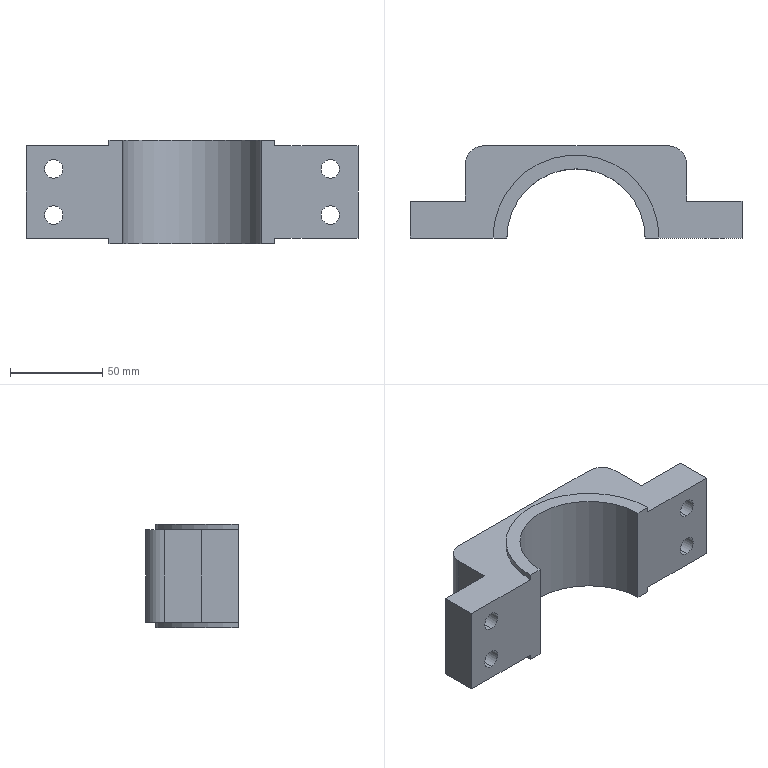Part | SolidWorks | features ICE 4, Extrusion 1, Fillet 1, MirrorPattern 1 | 1 solid | 26 faces | box 180 x 50 x 56 mm | volume 246956 mm3 | cylinder 13 | plane 13 | commonest cylinder face diameters 10 x8 20 x2 90 x2 75 x1
STEP:
#1=CARTESIAN_POINT('',(-75.,0.,17.5));
#2=VERTEX_POINT('',#1);
#3=CARTESIAN_POINT('',(-75.,0.,7.5));
#4=VERTEX_POINT('',#3);
#5=CARTESIAN_POINT('',(-75.,0.,12.5));
#6=DIRECTION('',(0.,-1.,0.));
#7=DIRECTION('',(0.,0.,-1.));
#8=AXIS2_PLACEMENT_3D('',#5,#6,#7);
#9=CIRCLE('',#8,5.);
#10=EDGE_CURVE('',#2,#4,#9,.T.);
#11=ORIENTED_EDGE('',*,*,#10,.T.);
#12=CARTESIAN_POINT('',(-75.,20.,7.5));
#13=VERTEX_POINT('',#12);
#14=CARTESIAN_POINT('',(-75.,-18.,7.5));
#15=DIRECTION('',(0.,1.,0.));
#16=VECTOR('',#15,1000.);
#17=LINE('',#14,#16);
#18=EDGE_CURVE('',#4,#13,#17,.T.);
#19=ORIENTED_EDGE('',*,*,#18,.T.);
#20=CARTESIAN_POINT('',(-75.,20.,17.5));
#21=VERTEX_POINT('',#20);
#22=CARTESIAN_POINT('',(-75.,20.,12.5));
#23=DIRECTION('',(0.,1.,0.));
#24=DIRECTION('',(0.,0.,1.));
#25=AXIS2_PLACEMENT_3D('',#22,#23,#24);
#26=CIRCLE('',#25,5.);
#27=EDGE_CURVE('',#13,#21,#26,.T.);
#28=ORIENTED_EDGE('',*,*,#27,.T.);
#29=CARTESIAN_POINT('',(-75.,-18.,17.5));
#30=DIRECTION('',(0.,1.,0.));
#31=VECTOR('',#30,1000.);
#32=LINE('',#29,#31);
#33=EDGE_CURVE('',#2,#21,#32,.T.);
#34=ORIENTED_EDGE('',*,*,#33,.F.);
#35=EDGE_LOOP('',(#11,#19,#28,#34));
#36=FACE_OUTER_BOUND('',#35,.T.);
#37=CARTESIAN_POINT('',(-75.,-18.,12.5));
#38=DIRECTION('',(0.,1.,0.));
#39=DIRECTION('',(0.,0.,1.));
#40=AXIS2_PLACEMENT_3D('',#37,#38,#39);
#41=CYLINDRICAL_SURFACE('',#40,5.);
#42=ADVANCED_FACE('',(#36),#41,.F.);
#43=CARTESIAN_POINT('',(-75.,0.,-7.5));
#44=VERTEX_POINT('',#43);
#45=CARTESIAN_POINT('',(-75.,0.,-17.5));
#46=VERTEX_POINT('',#45);
#47=CARTESIAN_POINT('',(-75.,0.,-12.5));
#48=DIRECTION('',(0.,-1.,0.));
#49=DIRECTION('',(0.,0.,-1.));
#50=AXIS2_PLACEMENT_3D('',#47,#48,#49);
#51=CIRCLE('',#50,5.);
#52=EDGE_CURVE('',#44,#46,#51,.T.);
#53=ORIENTED_EDGE('',*,*,#52,.T.);
#54=CARTESIAN_POINT('',(-75.,20.,-17.5));
#55=VERTEX_POINT('',#54);
#56=CARTESIAN_POINT('',(-75.,-18.,-17.5));
#57=DIRECTION('',(0.,1.,0.));
#58=VECTOR('',#57,1000.);
#59=LINE('',#56,#58);
#60=EDGE_CURVE('',#46,#55,#59,.T.);
#61=ORIENTED_EDGE('',*,*,#60,.T.);
#62=CARTESIAN_POINT('',(-75.,20.,-7.5));
#63=VERTEX_POINT('',#62);
#64=CARTESIAN_POINT('',(-75.,20.,-12.5));
#65=DIRECTION('',(0.,1.,0.));
#66=DIRECTION('',(0.,0.,1.));
#67=AXIS2_PLACEMENT_3D('',#64,#65,#66);
#68=CIRCLE('',#67,5.);
#69=EDGE_CURVE('',#55,#63,#68,.T.);
#70=ORIENTED_EDGE('',*,*,#69,.T.);
#71=CARTESIAN_POINT('',(-75.,-18.,-7.5));
#72=DIRECTION('',(0.,1.,0.));
#73=VECTOR('',#72,1000.);
#74=LINE('',#71,#73);
#75=EDGE_CURVE('',#44,#63,#74,.T.);
#76=ORIENTED_EDGE('',*,*,#75,.F.);
#77=EDGE_LOOP('',(#53,#61,#70,#76));
#78=FACE_OUTER_BOUND('',#77,.T.);
#79=CARTESIAN_POINT('',(-75.,-18.,-12.5));
#80=DIRECTION('',(0.,1.,0.));
#81=DIRECTION('',(0.,0.,1.));
#82=AXIS2_PLACEMENT_3D('',#79,#80,#81);
#83=CYLINDRICAL_SURFACE('',#82,5.);
#84=ADVANCED_FACE('',(#78),#83,.F.);
#85=CARTESIAN_POINT('',(75.,0.,-7.5));
#86=VERTEX_POINT('',#85);
#87=CARTESIAN_POINT('',(75.,0.,-17.5));
#88=VERTEX_POINT('',#87);
#89=CARTESIAN_POINT('',(75.,0.,-12.5));
#90=DIRECTION('',(0.,-1.,0.));
#91=DIRECTION('',(0.,0.,-1.));
#92=AXIS2_PLACEMENT_3D('',#89,#90,#91);
#93=CIRCLE('',#92,5.);
#94=EDGE_CURVE('',#86,#88,#93,.T.);
#95=ORIENTED_EDGE('',*,*,#94,.T.);
#96=CARTESIAN_POINT('',(75.,20.,-17.5));
#97=VERTEX_POINT('',#96);
#98=CARTESIAN_POINT('',(75.,-18.,-17.5));
#99=DIRECTION('',(0.,1.,0.));
#100=VECTOR('',#99,1000.);
#101=LINE('',#98,#100);
#102=EDGE_CURVE('',#88,#97,#101,.T.);
#103=ORIENTED_EDGE('',*,*,#102,.T.);
#104=CARTESIAN_POINT('',(75.,20.,-7.5));
#105=VERTEX_POINT('',#104);
#106=CARTESIAN_POINT('',(75.,20.,-12.5));
#107=DIRECTION('',(0.,1.,0.));
#108=DIRECTION('',(0.,0.,-1.));
#109=AXIS2_PLACEMENT_3D('',#106,#107,#108);
#110=CIRCLE('',#109,5.);
#111=EDGE_CURVE('',#97,#105,#110,.T.);
#112=ORIENTED_EDGE('',*,*,#111,.T.);
#113=CARTESIAN_POINT('',(75.,-18.,-7.5));
#114=DIRECTION('',(0.,1.,0.));
#115=VECTOR('',#114,1000.);
#116=LINE('',#113,#115);
#117=EDGE_CURVE('',#86,#105,#116,.T.);
#118=ORIENTED_EDGE('',*,*,#117,.F.);
#119=EDGE_LOOP('',(#95,#103,#112,#118));
#120=FACE_OUTER_BOUND('',#119,.T.);
#121=CARTESIAN_POINT('',(75.,-18.,-12.5));
#122=DIRECTION('',(0.,1.,0.));
#123=DIRECTION('',(0.,0.,1.));
#124=AXIS2_PLACEMENT_3D('',#121,#122,#123);
#125=CYLINDRICAL_SURFACE('',#124,5.);
#126=ADVANCED_FACE('',(#120),#125,.F.);
#127=CARTESIAN_POINT('',(75.,0.,17.5));
#128=VERTEX_POINT('',#127);
#129=CARTESIAN_POINT('',(75.,0.,7.5));
#130=VERTEX_POINT('',#129);
#131=CARTESIAN_POINT('',(75.,0.,12.5));
#132=DIRECTION('',(0.,-1.,0.));
#133=DIRECTION('',(0.,0.,-1.));
#134=AXIS2_PLACEMENT_3D('',#131,#132,#133);
#135=CIRCLE('',#134,5.);
#136=EDGE_CURVE('',#128,#130,#135,.T.);
#137=ORIENTED_EDGE('',*,*,#136,.T.);
#138=CARTESIAN_POINT('',(75.,20.,7.5));
#139=VERTEX_POINT('',#138);
#140=CARTESIAN_POINT('',(75.,-18.,7.5));
#141=DIRECTION('',(0.,1.,0.));
#142=VECTOR('',#141,1000.);
#143=LINE('',#140,#142);
#144=EDGE_CURVE('',#130,#139,#143,.T.);
#145=ORIENTED_EDGE('',*,*,#144,.T.);
#146=CARTESIAN_POINT('',(75.,20.,17.5));
#147=VERTEX_POINT('',#146);
#148=CARTESIAN_POINT('',(75.,20.,12.5));
#149=DIRECTION('',(0.,1.,0.));
#150=DIRECTION('',(0.,0.,-1.));
#151=AXIS2_PLACEMENT_3D('',#148,#149,#150);
#152=CIRCLE('',#151,5.);
#153=EDGE_CURVE('',#139,#147,#152,.T.);
#154=ORIENTED_EDGE('',*,*,#153,.T.);
#155=CARTESIAN_POINT('',(75.,-18.,17.5));
#156=DIRECTION('',(0.,1.,0.));
#157=VECTOR('',#156,1000.);
#158=LINE('',#155,#157);
#159=EDGE_CURVE('',#128,#147,#158,.T.);
#160=ORIENTED_EDGE('',*,*,#159,.F.);
#161=EDGE_LOOP('',(#137,#145,#154,#160));
#162=FACE_OUTER_BOUND('',#161,.T.);
#163=CARTESIAN_POINT('',(75.,-18.,12.5));
#164=DIRECTION('',(0.,1.,0.));
#165=DIRECTION('',(0.,0.,1.));
#166=AXIS2_PLACEMENT_3D('',#163,#164,#165);
#167=CYLINDRICAL_SURFACE('',#166,5.);
#168=ADVANCED_FACE('',(#162),#167,.F.);
#169=CARTESIAN_POINT('',(60.,20.,25.));
#170=VERTEX_POINT('',#169);
#171=CARTESIAN_POINT('',(60.,20.,-25.));
#172=VERTEX_POINT('',#171);
#173=CARTESIAN_POINT('',(60.,20.,25.));
#174=DIRECTION('',(0.,0.,-1.));
#175=VECTOR('',#174,1000.);
#176=LINE('',#173,#175);
#177=EDGE_CURVE('',#170,#172,#176,.T.);
#178=ORIENTED_EDGE('',*,*,#177,.T.);
#179=CARTESIAN_POINT('',(60.,40.,-25.));
#180=VERTEX_POINT('',#179);
#181=CARTESIAN_POINT('',(60.,50.,-25.));
#182=DIRECTION('',(0.,-1.,0.));
#183=VECTOR('',#182,1000.);
#184=LINE('',#181,#183);
#185=EDGE_CURVE('',#180,#172,#184,.T.);
#186=ORIENTED_EDGE('',*,*,#185,.F.);
#187=CARTESIAN_POINT('',(60.,40.,25.));
#188=VERTEX_POINT('',#187);
#189=CARTESIAN_POINT('',(60.,40.,25.));
#190=DIRECTION('',(0.,0.,1.));
#191=VECTOR('',#190,1000.);
#192=LINE('',#189,#191);
#193=EDGE_CURVE('',#180,#188,#192,.T.);
#194=ORIENTED_EDGE('',*,*,#193,.T.);
#195=CARTESIAN_POINT('',(60.,50.,25.));
#196=DIRECTION('',(0.,-1.,0.));
#197=VECTOR('',#196,1000.);
#198=LINE('',#195,#197);
#199=EDGE_CURVE('',#188,#170,#198,.T.);
#200=ORIENTED_EDGE('',*,*,#199,.T.);
#201=EDGE_LOOP('',(#178,#186,#194,#200));
#202=FACE_OUTER_BOUND('',#201,.T.);
#203=CARTESIAN_POINT('',(60.,50.,25.));
#204=DIRECTION('',(-1.,0.,0.));
#205=DIRECTION('',(0.,0.,1.));
#206=AXIS2_PLACEMENT_3D('',#203,#204,#205);
#207=PLANE('',#206);
#208=ADVANCED_FACE('',(#202),#207,.F.);
#209=ORIENTED_EDGE('',*,*,#94,.F.);
#210=CARTESIAN_POINT('',(75.,0.,-12.5));
#211=DIRECTION('',(0.,-1.,0.));
#212=DIRECTION('',(0.,0.,-1.));
#213=AXIS2_PLACEMENT_3D('',#210,#211,#212);
#214=CIRCLE('',#213,5.);
#215=EDGE_CURVE('',#88,#86,#214,.T.);
#216=ORIENTED_EDGE('',*,*,#215,.F.);
#217=EDGE_LOOP('',(#209,#216));
#218=FACE_BOUND('',#217,.T.);
#219=ORIENTED_EDGE('',*,*,#136,.F.);
#220=CARTESIAN_POINT('',(75.,0.,12.5));
#221=DIRECTION('',(0.,-1.,0.));
#222=DIRECTION('',(0.,0.,-1.));
#223=AXIS2_PLACEMENT_3D('',#220,#221,#222);
#224=CIRCLE('',#223,5.);
#225=EDGE_CURVE('',#130,#128,#224,.T.);
#226=ORIENTED_EDGE('',*,*,#225,.F.);
#227=EDGE_LOOP('',(#219,#226));
#228=FACE_BOUND('',#227,.T.);
#229=CARTESIAN_POINT('',(37.5,0.,-28.));
#230=VERTEX_POINT('',#229);
#231=CARTESIAN_POINT('',(37.5,0.,28.));
#232=VERTEX_POINT('',#231);
#233=CARTESIAN_POINT('',(37.5,0.,-114.));
#234=DIRECTION('',(0.,0.,1.));
#235=VECTOR('',#234,1000.);
#236=LINE('',#233,#235);
#237=EDGE_CURVE('',#230,#232,#236,.T.);
#238=ORIENTED_EDGE('',*,*,#237,.F.);
#239=CARTESIAN_POINT('',(45.,0.,-28.));
#240=VERTEX_POINT('',#239);
#241=CARTESIAN_POINT('',(37.5,0.,-28.));
#242=DIRECTION('',(1.,0.,0.));
#243=VECTOR('',#242,1000.);
#244=LINE('',#241,#243);
#245=EDGE_CURVE('',#230,#240,#244,.T.);
#246=ORIENTED_EDGE('',*,*,#245,.T.);
#247=CARTESIAN_POINT('',(45.,0.,-25.));
#248=VERTEX_POINT('',#247);
#249=CARTESIAN_POINT('',(45.,0.,-28.));
#250=DIRECTION('',(0.,0.,1.));
#251=VECTOR('',#250,1000.);
#252=LINE('',#249,#251);
#253=EDGE_CURVE('',#240,#248,#252,.T.);
#254=ORIENTED_EDGE('',*,*,#253,.T.);
#255=CARTESIAN_POINT('',(90.,0.,-25.));
#256=VERTEX_POINT('',#255);
#257=CARTESIAN_POINT('',(-60.,0.,-25.));
#258=DIRECTION('',(1.,0.,0.));
#259=VECTOR('',#258,1000.);
#260=LINE('',#257,#259);
#261=EDGE_CURVE('',#248,#256,#260,.T.);
#262=ORIENTED_EDGE('',*,*,#261,.T.);
#263=CARTESIAN_POINT('',(90.,0.,25.));
#264=VERTEX_POINT('',#263);
#265=CARTESIAN_POINT('',(90.,0.,-25.));
#266=DIRECTION('',(0.,0.,1.));
#267=VECTOR('',#266,1000.);
#268=LINE('',#265,#267);
#269=EDGE_CURVE('',#256,#264,#268,.T.);
#270=ORIENTED_EDGE('',*,*,#269,.T.);
#271=CARTESIAN_POINT('',(45.,0.,25.));
#272=VERTEX_POINT('',#271);
#273=CARTESIAN_POINT('',(-60.,0.,25.));
#274=DIRECTION('',(1.,0.,0.));
#275=VECTOR('',#274,1000.);
#276=LINE('',#273,#275);
#277=EDGE_CURVE('',#272,#264,#276,.T.);
#278=ORIENTED_EDGE('',*,*,#277,.F.);
#279=CARTESIAN_POINT('',(45.,0.,28.));
#280=VERTEX_POINT('',#279);
#281=CARTESIAN_POINT('',(45.,0.,28.));
#282=DIRECTION('',(0.,0.,-1.));
#283=VECTOR('',#282,1000.);
#284=LINE('',#281,#283);
#285=EDGE_CURVE('',#280,#272,#284,.T.);
#286=ORIENTED_EDGE('',*,*,#285,.F.);
#287=CARTESIAN_POINT('',(37.5,0.,28.));
#288=DIRECTION('',(1.,0.,0.));
#289=VECTOR('',#288,1000.);
#290=LINE('',#287,#289);
#291=EDGE_CURVE('',#232,#280,#290,.T.);
#292=ORIENTED_EDGE('',*,*,#291,.F.);
#293=EDGE_LOOP('',(#238,#246,#254,#262,#270,#278,#286,#292));
#294=FACE_OUTER_BOUND('',#293,.T.);
#295=CARTESIAN_POINT('',(0.,0.,0.));
#296=DIRECTION('',(0.,-1.,0.));
#297=DIRECTION('',(0.,0.,-1.));
#298=AXIS2_PLACEMENT_3D('',#295,#296,#297);
#299=PLANE('',#298);
#300=ADVANCED_FACE('',(#218,#228,#294),#299,.T.);
#301=CARTESIAN_POINT('',(-60.,20.,-25.));
#302=VERTEX_POINT('',#301);
#303=CARTESIAN_POINT('',(-60.,20.,25.));
#304=VERTEX_POINT('',#303);
#305=CARTESIAN_POINT('',(-60.,20.,25.));
#306=DIRECTION('',(0.,0.,1.));
#307=VECTOR('',#306,1000.);
#308=LINE('',#305,#307);
#309=EDGE_CURVE('',#302,#304,#308,.T.);
#310=ORIENTED_EDGE('',*,*,#309,.T.);
#311=CARTESIAN_POINT('',(-60.,40.,25.));
#312=VERTEX_POINT('',#311);
#313=CARTESIAN_POINT('',(-60.,50.,25.));
#314=DIRECTION('',(0.,-1.,0.));
#315=VECTOR('',#314,1000.);
#316=LINE('',#313,#315);
#317=EDGE_CURVE('',#312,#304,#316,.T.);
#318=ORIENTED_EDGE('',*,*,#317,.F.);
#319=CARTESIAN_POINT('',(-60.,40.,-25.));
#320=VERTEX_POINT('',#319);
#321=CARTESIAN_POINT('',(-60.,40.,-25.));
#322=DIRECTION('',(0.,0.,-1.));
#323=VECTOR('',#322,1000.);
#324=LINE('',#321,#323);
#325=EDGE_CURVE('',#312,#320,#324,.T.);
#326=ORIENTED_EDGE('',*,*,#325,.T.);
#327=CARTESIAN_POINT('',(-60.,50.,-25.));
#328=DIRECTION('',(0.,-1.,0.));
#329=VECTOR('',#328,1000.);
#330=LINE('',#327,#329);
#331=EDGE_CURVE('',#320,#302,#330,.T.);
#332=ORIENTED_EDGE('',*,*,#331,.T.);
#333=EDGE_LOOP('',(#310,#318,#326,#332));
#334=FACE_OUTER_BOUND('',#333,.T.);
#335=CARTESIAN_POINT('',(-60.,50.,25.));
#336=DIRECTION('',(-1.,0.,0.));
#337=DIRECTION('',(0.,0.,1.));
#338=AXIS2_PLACEMENT_3D('',#335,#336,#337);
#339=PLANE('',#338);
#340=ADVANCED_FACE('',(#334),#339,.T.);
#341=CARTESIAN_POINT('',(-45.,0.,25.));
#342=VERTEX_POINT('',#341);
#343=CARTESIAN_POINT('',(0.,0.,25.));
#344=DIRECTION('',(0.,0.,1.));
#345=DIRECTION('',(1.,0.,0.));
#346=AXIS2_PLACEMENT_3D('',#343,#344,#345);
#347=CIRCLE('',#346,45.);
#348=EDGE_CURVE('',#272,#342,#347,.T.);
#349=ORIENTED_EDGE('',*,*,#348,.F.);
#350=ORIENTED_EDGE('',*,*,#277,.T.);
#351=CARTESIAN_POINT('',(90.,20.,25.));
#352=VERTEX_POINT('',#351);
#353=CARTESIAN_POINT('',(90.,20.,25.));
#354=DIRECTION('',(0.,-1.,0.));
#355=VECTOR('',#354,1000.);
#356=LINE('',#353,#355);
#357=EDGE_CURVE('',#352,#264,#356,.T.);
#358=ORIENTED_EDGE('',*,*,#357,.F.);
#359=CARTESIAN_POINT('',(60.,20.,25.));
#360=DIRECTION('',(-1.,0.,0.));
#361=VECTOR('',#360,1000.);
#362=LINE('',#359,#361);
#363=EDGE_CURVE('',#352,#170,#362,.T.);
#364=ORIENTED_EDGE('',*,*,#363,.T.);
#365=ORIENTED_EDGE('',*,*,#199,.F.);
#366=CARTESIAN_POINT('',(50.,50.,25.));
#367=VERTEX_POINT('',#366);
#368=CARTESIAN_POINT('',(50.,40.,25.));
#369=DIRECTION('',(0.,0.,1.));
#370=DIRECTION('',(-1.,0.,0.));
#371=AXIS2_PLACEMENT_3D('',#368,#369,#370);
#372=CIRCLE('',#371,10.);
#373=EDGE_CURVE('',#188,#367,#372,.T.);
#374=ORIENTED_EDGE('',*,*,#373,.T.);
#375=CARTESIAN_POINT('',(-50.,50.,25.));
#376=VERTEX_POINT('',#375);
#377=CARTESIAN_POINT('',(-60.,50.,25.));
#378=DIRECTION('',(1.,0.,0.));
#379=VECTOR('',#378,1000.);
#380=LINE('',#377,#379);
#381=EDGE_CURVE('',#376,#367,#380,.T.);
#382=ORIENTED_EDGE('',*,*,#381,.F.);
#383=CARTESIAN_POINT('',(-50.,40.,25.));
#384=DIRECTION('',(0.,0.,1.));
#385=DIRECTION('',(-1.,0.,0.));
#386=AXIS2_PLACEMENT_3D('',#383,#384,#385);
#387=CIRCLE('',#386,10.);
#388=EDGE_CURVE('',#376,#312,#387,.T.);
#389=ORIENTED_EDGE('',*,*,#388,.T.);
#390=ORIENTED_EDGE('',*,*,#317,.T.);
#391=CARTESIAN_POINT('',(-90.,20.,25.));
#392=VERTEX_POINT('',#391);
#393=CARTESIAN_POINT('',(-90.,20.,25.));
#394=DIRECTION('',(-1.,0.,0.));
#395=VECTOR('',#394,1000.);
#396=LINE('',#393,#395);
#397=EDGE_CURVE('',#304,#392,#396,.T.);
#398=ORIENTED_EDGE('',*,*,#397,.T.);
#399=CARTESIAN_POINT('',(-90.,0.,25.));
#400=VERTEX_POINT('',#399);
#401=CARTESIAN_POINT('',(-90.,20.,25.));
#402=DIRECTION('',(0.,-1.,0.));
#403=VECTOR('',#402,1000.);
#404=LINE('',#401,#403);
#405=EDGE_CURVE('',#392,#400,#404,.T.);
#406=ORIENTED_EDGE('',*,*,#405,.T.);
#407=CARTESIAN_POINT('',(-60.,0.,25.));
#408=DIRECTION('',(1.,0.,0.));
#409=VECTOR('',#408,1000.);
#410=LINE('',#407,#409);
#411=EDGE_CURVE('',#400,#342,#410,.T.);
#412=ORIENTED_EDGE('',*,*,#411,.T.);
#413=EDGE_LOOP('',(#349,#350,#358,#364,#365,#374,#382,#389,#390,#398,#406,#412));
#414=FACE_OUTER_BOUND('',#413,.T.);
#415=CARTESIAN_POINT('',(-60.,50.,25.));
#416=DIRECTION('',(0.,0.,-1.));
#417=DIRECTION('',(-1.,0.,0.));
#418=AXIS2_PLACEMENT_3D('',#415,#416,#417);
#419=PLANE('',#418);
#420=ADVANCED_FACE('',(#414),#419,.F.);
#421=ORIENTED_EDGE('',*,*,#261,.F.);
#422=CARTESIAN_POINT('',(-45.,0.,-25.));
#423=VERTEX_POINT('',#422);
#424=CARTESIAN_POINT('',(0.,0.,-25.));
#425=DIRECTION('',(0.,0.,1.));
#426=DIRECTION('',(1.,0.,0.));
#427=AXIS2_PLACEMENT_3D('',#424,#425,#426);
#428=CIRCLE('',#427,45.);
#429=EDGE_CURVE('',#248,#423,#428,.T.);
#430=ORIENTED_EDGE('',*,*,#429,.T.);
#431=CARTESIAN_POINT('',(-90.,0.,-25.));
#432=VERTEX_POINT('',#431);
#433=CARTESIAN_POINT('',(-60.,0.,-25.));
#434=DIRECTION('',(1.,0.,0.));
#435=VECTOR('',#434,1000.);
#436=LINE('',#433,#435);
#437=EDGE_CURVE('',#432,#423,#436,.T.);
#438=ORIENTED_EDGE('',*,*,#437,.F.);
#439=CARTESIAN_POINT('',(-90.,20.,-25.));
#440=VERTEX_POINT('',#439);
#441=CARTESIAN_POINT('',(-90.,20.,-25.));
#442=DIRECTION('',(0.,-1.,0.));
#443=VECTOR('',#442,1000.);
#444=LINE('',#441,#443);
#445=EDGE_CURVE('',#440,#432,#444,.T.);
#446=ORIENTED_EDGE('',*,*,#445,.F.);
#447=CARTESIAN_POINT('',(-90.,20.,-25.));
#448=DIRECTION('',(1.,0.,0.));
#449=VECTOR('',#448,1000.);
#450=LINE('',#447,#449);
#451=EDGE_CURVE('',#440,#302,#450,.T.);
#452=ORIENTED_EDGE('',*,*,#451,.T.);
#453=ORIENTED_EDGE('',*,*,#331,.F.);
#454=CARTESIAN_POINT('',(-50.,50.,-25.));
#455=VERTEX_POINT('',#454);
#456=CARTESIAN_POINT('',(-50.,40.,-25.));
#457=DIRECTION('',(0.,0.,-1.));
#458=DIRECTION('',(-1.,0.,0.));
#459=AXIS2_PLACEMENT_3D('',#456,#457,#458);
#460=CIRCLE('',#459,10.);
#461=EDGE_CURVE('',#320,#455,#460,.T.);
#462=ORIENTED_EDGE('',*,*,#461,.T.);
#463=CARTESIAN_POINT('',(50.,50.,-25.));
#464=VERTEX_POINT('',#463);
#465=CARTESIAN_POINT('',(-60.,50.,-25.));
#466=DIRECTION('',(1.,0.,0.));
#467=VECTOR('',#466,1000.);
#468=LINE('',#465,#467);
#469=EDGE_CURVE('',#455,#464,#468,.T.);
#470=ORIENTED_EDGE('',*,*,#469,.T.);
#471=CARTESIAN_POINT('',(50.,40.,-25.));
#472=DIRECTION('',(0.,0.,-1.));
#473=DIRECTION('',(-1.,0.,0.));
#474=AXIS2_PLACEMENT_3D('',#471,#472,#473);
#475=CIRCLE('',#474,10.);
#476=EDGE_CURVE('',#464,#180,#475,.T.);
#477=ORIENTED_EDGE('',*,*,#476,.T.);
#478=ORIENTED_EDGE('',*,*,#185,.T.);
#479=CARTESIAN_POINT('',(90.,20.,-25.));
#480=VERTEX_POINT('',#479);
#481=CARTESIAN_POINT('',(60.,20.,-25.));
#482=DIRECTION('',(1.,0.,0.));
#483=VECTOR('',#482,1000.);
#484=LINE('',#481,#483);
#485=EDGE_CURVE('',#172,#480,#484,.T.);
#486=ORIENTED_EDGE('',*,*,#485,.T.);
#487=CARTESIAN_POINT('',(90.,20.,-25.));
#488=DIRECTION('',(0.,-1.,0.));
#489=VECTOR('',#488,1000.);
#490=LINE('',#487,#489);
#491=EDGE_CURVE('',#480,#256,#490,.T.);
#492=ORIENTED_EDGE('',*,*,#491,.T.);
#493=EDGE_LOOP('',(#421,#430,#438,#446,#452,#453,#462,#470,#477,#478,#486,#492));
#494=FACE_OUTER_BOUND('',#493,.T.);
#495=CARTESIAN_POINT('',(-60.,50.,-25.));
#496=DIRECTION('',(0.,0.,-1.));
#497=DIRECTION('',(-1.,0.,0.));
#498=AXIS2_PLACEMENT_3D('',#495,#496,#497);
#499=PLANE('',#498);
#500=ADVANCED_FACE('',(#494),#499,.T.);
#501=ORIENTED_EDGE('',*,*,#381,.T.);
#502=CARTESIAN_POINT('',(50.,50.,0.));
#503=DIRECTION('',(0.,0.,-1.));
#504=VECTOR('',#503,1000.);
#505=LINE('',#502,#504);
#506=EDGE_CURVE('',#367,#464,#505,.T.);
#507=ORIENTED_EDGE('',*,*,#506,.T.);
#508=ORIENTED_EDGE('',*,*,#469,.F.);
#509=CARTESIAN_POINT('',(-50.,50.,25.));
#510=DIRECTION('',(0.,0.,1.));
#511=VECTOR('',#510,1000.);
#512=LINE('',#509,#511);
#513=EDGE_CURVE('',#455,#376,#512,.T.);
#514=ORIENTED_EDGE('',*,*,#513,.T.);
#515=EDGE_LOOP('',(#501,#507,#508,#514));
#516=FACE_OUTER_BOUND('',#515,.T.);
#517=CARTESIAN_POINT('',(0.,50.,0.));
#518=DIRECTION('',(0.,-1.,0.));
#519=DIRECTION('',(0.,0.,-1.));
#520=AXIS2_PLACEMENT_3D('',#517,#518,#519);
#521=PLANE('',#520);
#522=ADVANCED_FACE('',(#516),#521,.F.);
#523=ORIENTED_EDGE('',*,*,#10,.F.);
#524=CARTESIAN_POINT('',(-75.,0.,12.5));
#525=DIRECTION('',(0.,-1.,0.));
#526=DIRECTION('',(0.,0.,-1.));
#527=AXIS2_PLACEMENT_3D('',#524,#525,#526);
#528=CIRCLE('',#527,5.);
#529=EDGE_CURVE('',#4,#2,#528,.T.);
#530=ORIENTED_EDGE('',*,*,#529,.F.);
#531=EDGE_LOOP('',(#523,#530));
#532=FACE_BOUND('',#531,.T.);
#533=ORIENTED_EDGE('',*,*,#52,.F.);
#534=CARTESIAN_POINT('',(-75.,0.,-12.5));
#535=DIRECTION('',(0.,-1.,0.));
#536=DIRECTION('',(0.,0.,-1.));
#537=AXIS2_PLACEMENT_3D('',#534,#535,#536);
#538=CIRCLE('',#537,5.);
#539=EDGE_CURVE('',#46,#44,#538,.T.);
#540=ORIENTED_EDGE('',*,*,#539,.F.);
#541=EDGE_LOOP('',(#533,#540));
#542=FACE_BOUND('',#541,.T.);
#543=CARTESIAN_POINT('',(-37.5,0.,28.));
#544=VERTEX_POINT('',#543);
#545=CARTESIAN_POINT('',(-37.5,0.,-28.));
#546=VERTEX_POINT('',#545);
#547=CARTESIAN_POINT('',(-37.5,0.,-114.));
#548=DIRECTION('',(0.,0.,-1.));
#549=VECTOR('',#548,1000.);
#550=LINE('',#547,#549);
#551=EDGE_CURVE('',#544,#546,#550,.T.);
#552=ORIENTED_EDGE('',*,*,#551,.F.);
#553=CARTESIAN_POINT('',(-45.,0.,28.));
#554=VERTEX_POINT('',#553);
#555=CARTESIAN_POINT('',(-45.,0.,28.));
#556=DIRECTION('',(1.,0.,0.));
#557=VECTOR('',#556,1000.);
#558=LINE('',#555,#557);
#559=EDGE_CURVE('',#554,#544,#558,.T.);
#560=ORIENTED_EDGE('',*,*,#559,.F.);
#561=CARTESIAN_POINT('',(-45.,0.,28.));
#562=DIRECTION('',(0.,0.,-1.));
#563=VECTOR('',#562,1000.);
#564=LINE('',#561,#563);
#565=EDGE_CURVE('',#554,#342,#564,.T.);
#566=ORIENTED_EDGE('',*,*,#565,.T.);
#567=ORIENTED_EDGE('',*,*,#411,.F.);
#568=CARTESIAN_POINT('',(-90.,0.,-25.));
#569=DIRECTION('',(0.,0.,-1.));
#570=VECTOR('',#569,1000.);
#571=LINE('',#568,#570);
#572=EDGE_CURVE('',#400,#432,#571,.T.);
#573=ORIENTED_EDGE('',*,*,#572,.T.);
#574=ORIENTED_EDGE('',*,*,#437,.T.);
#575=CARTESIAN_POINT('',(-45.,0.,-28.));
#576=VERTEX_POINT('',#575);
#577=CARTESIAN_POINT('',(-45.,0.,-28.));
#578=DIRECTION('',(0.,0.,1.));
#579=VECTOR('',#578,1000.);
#580=LINE('',#577,#579);
#581=EDGE_CURVE('',#576,#423,#580,.T.);
#582=ORIENTED_EDGE('',*,*,#581,.F.);
#583=CARTESIAN_POINT('',(-45.,0.,-28.));
#584=DIRECTION('',(1.,0.,0.));
#585=VECTOR('',#584,1000.);
#586=LINE('',#583,#585);
#587=EDGE_CURVE('',#576,#546,#586,.T.);
#588=ORIENTED_EDGE('',*,*,#587,.T.);
#589=EDGE_LOOP('',(#552,#560,#566,#567,#573,#574,#582,#588));
#590=FACE_OUTER_BOUND('',#589,.T.);
#591=CARTESIAN_POINT('',(0.,0.,0.));
#592=DIRECTION('',(0.,-1.,0.));
#593=DIRECTION('',(0.,0.,-1.));
#594=AXIS2_PLACEMENT_3D('',#591,#592,#593);
#595=PLANE('',#594);
#596=ADVANCED_FACE('',(#532,#542,#590),#595,.T.);
#597=ORIENTED_EDGE('',*,*,#237,.T.);
#598=CARTESIAN_POINT('',(0.,0.,28.));
#599=DIRECTION('',(0.,0.,-1.));
#600=DIRECTION('',(1.,0.,0.));
#601=AXIS2_PLACEMENT_3D('',#598,#599,#600);
#602=CIRCLE('',#601,37.5);
#603=EDGE_CURVE('',#544,#232,#602,.T.);
#604=ORIENTED_EDGE('',*,*,#603,.F.);
#605=ORIENTED_EDGE('',*,*,#551,.T.);
#606=CARTESIAN_POINT('',(0.,0.,-28.));
#607=DIRECTION('',(0.,0.,-1.));
#608=DIRECTION('',(1.,0.,0.));
#609=AXIS2_PLACEMENT_3D('',#606,#607,#608);
#610=CIRCLE('',#609,37.5);
#611=EDGE_CURVE('',#546,#230,#610,.T.);
#612=ORIENTED_EDGE('',*,*,#611,.T.);
#613=EDGE_LOOP('',(#597,#604,#605,#612));
#614=FACE_OUTER_BOUND('',#613,.T.);
#615=CARTESIAN_POINT('',(0.,0.,-114.));
#616=DIRECTION('',(0.,0.,1.));
#617=DIRECTION('',(1.,0.,0.));
#618=AXIS2_PLACEMENT_3D('',#615,#616,#617);
#619=CYLINDRICAL_SURFACE('',#618,37.5);
#620=ADVANCED_FACE('',(#614),#619,.F.);
#621=ORIENTED_EDGE('',*,*,#373,.F.);
#622=ORIENTED_EDGE('',*,*,#193,.F.);
#623=ORIENTED_EDGE('',*,*,#476,.F.);
#624=ORIENTED_EDGE('',*,*,#506,.F.);
#625=EDGE_LOOP('',(#621,#622,#623,#624));
#626=FACE_OUTER_BOUND('',#625,.T.);
#627=CARTESIAN_POINT('',(50.,40.,0.));
#628=DIRECTION('',(0.,0.,-1.));
#629=DIRECTION('',(-1.,0.,0.));
#630=AXIS2_PLACEMENT_3D('',#627,#628,#629);
#631=CYLINDRICAL_SURFACE('',#630,10.);
#632=ADVANCED_FACE('',(#626),#631,.T.);
#633=ORIENTED_EDGE('',*,*,#388,.F.);
#634=ORIENTED_EDGE('',*,*,#513,.F.);
#635=ORIENTED_EDGE('',*,*,#461,.F.);
#636=ORIENTED_EDGE('',*,*,#325,.F.);
#637=EDGE_LOOP('',(#633,#634,#635,#636));
#638=FACE_OUTER_BOUND('',#637,.T.);
#639=CARTESIAN_POINT('',(-50.,40.,25.));
#640=DIRECTION('',(0.,0.,1.));
#641=DIRECTION('',(1.,0.,0.));
#642=AXIS2_PLACEMENT_3D('',#639,#640,#641);
#643=CYLINDRICAL_SURFACE('',#642,10.);
#644=ADVANCED_FACE('',(#638),#643,.T.);
#645=ORIENTED_EDGE('',*,*,#572,.F.);
#646=ORIENTED_EDGE('',*,*,#405,.F.);
#647=CARTESIAN_POINT('',(-90.,20.,-25.));
#648=DIRECTION('',(0.,0.,-1.));
#649=VECTOR('',#648,1000.);
#650=LINE('',#647,#649);
#651=EDGE_CURVE('',#392,#440,#650,.T.);
#652=ORIENTED_EDGE('',*,*,#651,.T.);
#653=ORIENTED_EDGE('',*,*,#445,.T.);
#654=EDGE_LOOP('',(#645,#646,#652,#653));
#655=FACE_OUTER_BOUND('',#654,.T.);
#656=CARTESIAN_POINT('',(-90.,20.,-25.));
#657=DIRECTION('',(-1.,0.,0.));
#658=DIRECTION('',(0.,0.,1.));
#659=AXIS2_PLACEMENT_3D('',#656,#657,#658);
#660=PLANE('',#659);
#661=ADVANCED_FACE('',(#655),#660,.T.);
#662=CARTESIAN_POINT('',(-75.,20.,12.5));
#663=DIRECTION('',(0.,1.,0.));
#664=DIRECTION('',(0.,0.,1.));
#665=AXIS2_PLACEMENT_3D('',#662,#663,#664);
#666=CIRCLE('',#665,5.);
#667=EDGE_CURVE('',#21,#13,#666,.T.);
#668=ORIENTED_EDGE('',*,*,#667,.F.);
#669=ORIENTED_EDGE('',*,*,#27,.F.);
#670=EDGE_LOOP('',(#668,#669));
#671=FACE_BOUND('',#670,.T.);
#672=CARTESIAN_POINT('',(-75.,20.,-12.5));
#673=DIRECTION('',(0.,1.,0.));
#674=DIRECTION('',(0.,0.,1.));
#675=AXIS2_PLACEMENT_3D('',#672,#673,#674);
#676=CIRCLE('',#675,5.);
#677=EDGE_CURVE('',#63,#55,#676,.T.);
#678=ORIENTED_EDGE('',*,*,#677,.F.);
#679=ORIENTED_EDGE('',*,*,#69,.F.);
#680=EDGE_LOOP('',(#678,#679));
#681=FACE_BOUND('',#680,.T.);
#682=ORIENTED_EDGE('',*,*,#651,.F.);
#683=ORIENTED_EDGE('',*,*,#397,.F.);
#684=ORIENTED_EDGE('',*,*,#309,.F.);
#685=ORIENTED_EDGE('',*,*,#451,.F.);
#686=EDGE_LOOP('',(#682,#683,#684,#685));
#687=FACE_OUTER_BOUND('',#686,.T.);
#688=CARTESIAN_POINT('',(0.,20.,0.));
#689=DIRECTION('',(0.,1.,0.));
#690=DIRECTION('',(0.,0.,1.));
#691=AXIS2_PLACEMENT_3D('',#688,#689,#690);
#692=PLANE('',#691);
#693=ADVANCED_FACE('',(#671,#681,#687),#692,.T.);
#694=ORIENTED_EDGE('',*,*,#269,.F.);
#695=ORIENTED_EDGE('',*,*,#491,.F.);
#696=CARTESIAN_POINT('',(90.,20.,-25.));
#697=DIRECTION('',(0.,0.,1.));
#698=VECTOR('',#697,1000.);
#699=LINE('',#696,#698);
#700=EDGE_CURVE('',#480,#352,#699,.T.);
#701=ORIENTED_EDGE('',*,*,#700,.T.);
#702=ORIENTED_EDGE('',*,*,#357,.T.);
#703=EDGE_LOOP('',(#694,#695,#701,#702));
#704=FACE_OUTER_BOUND('',#703,.T.);
#705=CARTESIAN_POINT('',(90.,20.,-25.));
#706=DIRECTION('',(1.,0.,0.));
#707=DIRECTION('',(0.,0.,-1.));
#708=AXIS2_PLACEMENT_3D('',#705,#706,#707);
#709=PLANE('',#708);
#710=ADVANCED_FACE('',(#704),#709,.T.);
#711=CARTESIAN_POINT('',(75.,20.,-12.5));
#712=DIRECTION('',(0.,1.,0.));
#713=DIRECTION('',(0.,0.,-1.));
#714=AXIS2_PLACEMENT_3D('',#711,#712,#713);
#715=CIRCLE('',#714,5.);
#716=EDGE_CURVE('',#105,#97,#715,.T.);
#717=ORIENTED_EDGE('',*,*,#716,.F.);
#718=ORIENTED_EDGE('',*,*,#111,.F.);
#719=EDGE_LOOP('',(#717,#718));
#720=FACE_BOUND('',#719,.T.);
#721=CARTESIAN_POINT('',(75.,20.,12.5));
#722=DIRECTION('',(0.,1.,0.));
#723=DIRECTION('',(0.,0.,-1.));
#724=AXIS2_PLACEMENT_3D('',#721,#722,#723);
#725=CIRCLE('',#724,5.);
#726=EDGE_CURVE('',#147,#139,#725,.T.);
#727=ORIENTED_EDGE('',*,*,#726,.F.);
#728=ORIENTED_EDGE('',*,*,#153,.F.);
#729=EDGE_LOOP('',(#727,#728));
#730=FACE_BOUND('',#729,.T.);
#731=ORIENTED_EDGE('',*,*,#363,.F.);
#732=ORIENTED_EDGE('',*,*,#700,.F.);
#733=ORIENTED_EDGE('',*,*,#485,.F.);
#734=ORIENTED_EDGE('',*,*,#177,.F.);
#735=EDGE_LOOP('',(#731,#732,#733,#734));
#736=FACE_OUTER_BOUND('',#735,.T.);
#737=CARTESIAN_POINT('',(0.,20.,0.));
#738=DIRECTION('',(0.,-1.,0.));
#739=DIRECTION('',(0.,0.,-1.));
#740=AXIS2_PLACEMENT_3D('',#737,#738,#739);
#741=PLANE('',#740);
#742=ADVANCED_FACE('',(#720,#730,#736),#741,.F.);
#743=ORIENTED_EDGE('',*,*,#348,.T.);
#744=ORIENTED_EDGE('',*,*,#565,.F.);
#745=CARTESIAN_POINT('',(0.,0.,28.));
#746=DIRECTION('',(0.,0.,1.));
#747=DIRECTION('',(1.,0.,0.));
#748=AXIS2_PLACEMENT_3D('',#745,#746,#747);
#749=CIRCLE('',#748,45.);
#750=EDGE_CURVE('',#280,#554,#749,.T.);
#751=ORIENTED_EDGE('',*,*,#750,.F.);
#752=ORIENTED_EDGE('',*,*,#285,.T.);
#753=EDGE_LOOP('',(#743,#744,#751,#752));
#754=FACE_OUTER_BOUND('',#753,.T.);
#755=CARTESIAN_POINT('',(0.,0.,28.));
#756=DIRECTION('',(0.,0.,-1.));
#757=DIRECTION('',(-1.,0.,0.));
#758=AXIS2_PLACEMENT_3D('',#755,#756,#757);
#759=CYLINDRICAL_SURFACE('',#758,45.);
#760=ADVANCED_FACE('',(#754),#759,.T.);
#761=ORIENTED_EDGE('',*,*,#603,.T.);
#762=ORIENTED_EDGE('',*,*,#291,.T.);
#763=ORIENTED_EDGE('',*,*,#750,.T.);
#764=ORIENTED_EDGE('',*,*,#559,.T.);
#765=EDGE_LOOP('',(#761,#762,#763,#764));
#766=FACE_OUTER_BOUND('',#765,.T.);
#767=CARTESIAN_POINT('',(0.,0.,28.));
#768=DIRECTION('',(0.,0.,1.));
#769=DIRECTION('',(1.,0.,0.));
#770=AXIS2_PLACEMENT_3D('',#767,#768,#769);
#771=PLANE('',#770);
#772=ADVANCED_FACE('',(#766),#771,.T.);
#773=ORIENTED_EDGE('',*,*,#429,.F.);
#774=ORIENTED_EDGE('',*,*,#253,.F.);
#775=CARTESIAN_POINT('',(0.,0.,-28.));
#776=DIRECTION('',(0.,0.,1.));
#777=DIRECTION('',(1.,0.,0.));
#778=AXIS2_PLACEMENT_3D('',#775,#776,#777);
#779=CIRCLE('',#778,45.);
#780=EDGE_CURVE('',#240,#576,#779,.T.);
#781=ORIENTED_EDGE('',*,*,#780,.T.);
#782=ORIENTED_EDGE('',*,*,#581,.T.);
#783=EDGE_LOOP('',(#773,#774,#781,#782));
#784=FACE_OUTER_BOUND('',#783,.T.);
#785=CARTESIAN_POINT('',(0.,0.,-28.));
#786=DIRECTION('',(0.,0.,1.));
#787=DIRECTION('',(1.,0.,0.));
#788=AXIS2_PLACEMENT_3D('',#785,#786,#787);
#789=CYLINDRICAL_SURFACE('',#788,45.);
#790=ADVANCED_FACE('',(#784),#789,.T.);
#791=ORIENTED_EDGE('',*,*,#611,.F.);
#792=ORIENTED_EDGE('',*,*,#587,.F.);
#793=ORIENTED_EDGE('',*,*,#780,.F.);
#794=ORIENTED_EDGE('',*,*,#245,.F.);
#795=EDGE_LOOP('',(#791,#792,#793,#794));
#796=FACE_OUTER_BOUND('',#795,.T.);
#797=CARTESIAN_POINT('',(0.,0.,-28.));
#798=DIRECTION('',(0.,0.,-1.));
#799=DIRECTION('',(1.,0.,0.));
#800=AXIS2_PLACEMENT_3D('',#797,#798,#799);
#801=PLANE('',#800);
#802=ADVANCED_FACE('',(#796),#801,.T.);
#803=ORIENTED_EDGE('',*,*,#144,.F.);
#804=ORIENTED_EDGE('',*,*,#225,.T.);
#805=ORIENTED_EDGE('',*,*,#159,.T.);
#806=ORIENTED_EDGE('',*,*,#726,.T.);
#807=EDGE_LOOP('',(#803,#804,#805,#806));
#808=FACE_OUTER_BOUND('',#807,.T.);
#809=CARTESIAN_POINT('',(75.,-18.,12.5));
#810=DIRECTION('',(0.,1.,0.));
#811=DIRECTION('',(0.,0.,1.));
#812=AXIS2_PLACEMENT_3D('',#809,#810,#811);
#813=CYLINDRICAL_SURFACE('',#812,5.);
#814=ADVANCED_FACE('',(#808),#813,.F.);
#815=ORIENTED_EDGE('',*,*,#102,.F.);
#816=ORIENTED_EDGE('',*,*,#215,.T.);
#817=ORIENTED_EDGE('',*,*,#117,.T.);
#818=ORIENTED_EDGE('',*,*,#716,.T.);
#819=EDGE_LOOP('',(#815,#816,#817,#818));
#820=FACE_OUTER_BOUND('',#819,.T.);
#821=CARTESIAN_POINT('',(75.,-18.,-12.5));
#822=DIRECTION('',(0.,1.,0.));
#823=DIRECTION('',(0.,0.,1.));
#824=AXIS2_PLACEMENT_3D('',#821,#822,#823);
#825=CYLINDRICAL_SURFACE('',#824,5.);
#826=ADVANCED_FACE('',(#820),#825,.F.);
#827=ORIENTED_EDGE('',*,*,#60,.F.);
#828=ORIENTED_EDGE('',*,*,#539,.T.);
#829=ORIENTED_EDGE('',*,*,#75,.T.);
#830=ORIENTED_EDGE('',*,*,#677,.T.);
#831=EDGE_LOOP('',(#827,#828,#829,#830));
#832=FACE_OUTER_BOUND('',#831,.T.);
#833=CARTESIAN_POINT('',(-75.,-18.,-12.5));
#834=DIRECTION('',(0.,1.,0.));
#835=DIRECTION('',(0.,0.,1.));
#836=AXIS2_PLACEMENT_3D('',#833,#834,#835);
#837=CYLINDRICAL_SURFACE('',#836,5.);
#838=ADVANCED_FACE('',(#832),#837,.F.);
#839=ORIENTED_EDGE('',*,*,#18,.F.);
#840=ORIENTED_EDGE('',*,*,#529,.T.);
#841=ORIENTED_EDGE('',*,*,#33,.T.);
#842=ORIENTED_EDGE('',*,*,#667,.T.);
#843=EDGE_LOOP('',(#839,#840,#841,#842));
#844=FACE_OUTER_BOUND('',#843,.T.);
#845=CARTESIAN_POINT('',(-75.,-18.,12.5));
#846=DIRECTION('',(0.,1.,0.));
#847=DIRECTION('',(0.,0.,1.));
#848=AXIS2_PLACEMENT_3D('',#845,#846,#847);
#849=CYLINDRICAL_SURFACE('',#848,5.);
#850=ADVANCED_FACE('',(#844),#849,.F.);
#851=CLOSED_SHELL('',(#42,#84,#126,#168,#208,#300,#340,#420,#500,#522,#596,#620,#632,#644,#661,#693,#710,#742,#760,#772,#790,#802,#814,#826,#838,#850));
#852=MANIFOLD_SOLID_BREP('',#851);
#853=CARTESIAN_POINT('',(0.,0.,0.));
#854=DIRECTION('',(0.,0.,1.));
#855=DIRECTION('',(1.,0.,0.));
#856=AXIS2_PLACEMENT_3D('',#853,#854,#855);
#857=(LENGTH_UNIT()NAMED_UNIT(*)SI_UNIT(.MILLI.,.METRE.));
#858=UNCERTAINTY_MEASURE_WITH_UNIT(LENGTH_MEASURE(0.00001),#857,'','');
#859=(NAMED_UNIT(*)PLANE_ANGLE_UNIT()SI_UNIT($,.RADIAN.));
#860=(NAMED_UNIT(*)SI_UNIT($,.STERADIAN.)SOLID_ANGLE_UNIT());
#861=(GEOMETRIC_REPRESENTATION_CONTEXT(3)GLOBAL_UNCERTAINTY_ASSIGNED_CONTEXT((#858))GLOBAL_UNIT_ASSIGNED_CONTEXT((#857,#859,#860))REPRESENTATION_CONTEXT('',''));
#862=ADVANCED_BREP_SHAPE_REPRESENTATION('',(#852,#856),#861);